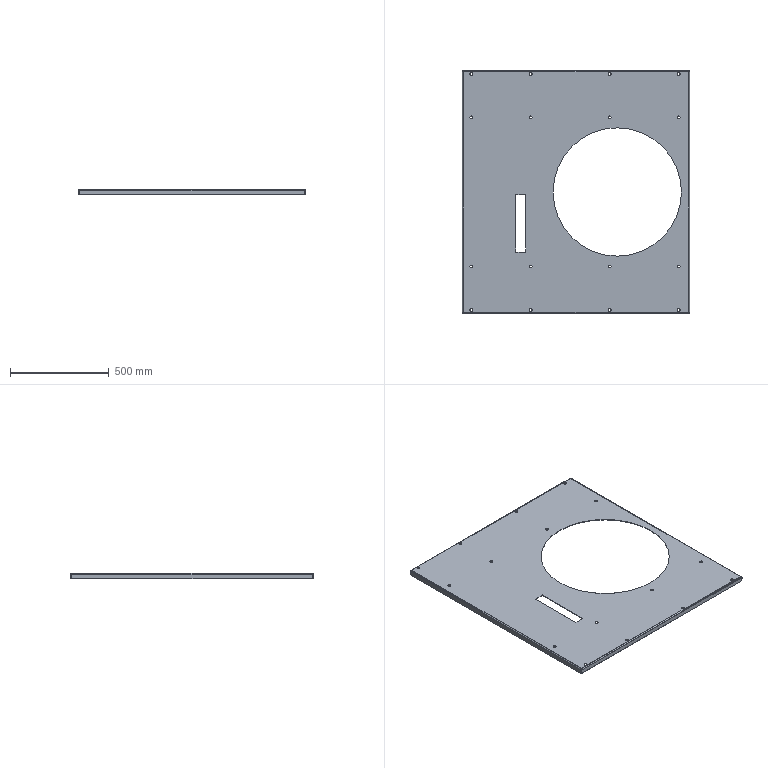Part | SolidWorks | features EdgeFlange 3, ICE 2, Extrusion 1, FlatPattern 1, HoleWzd 1, SheetMetal 1, SolidToSheetMetal 1 | 1 solid | 84 faces | box 1150 x 1228 x 28 mm | volume 3516679 mm3 | cylinder 42 | plane 42 | commonest cylinder face diameters 15 x32 6 x4 12 x4 650 x2